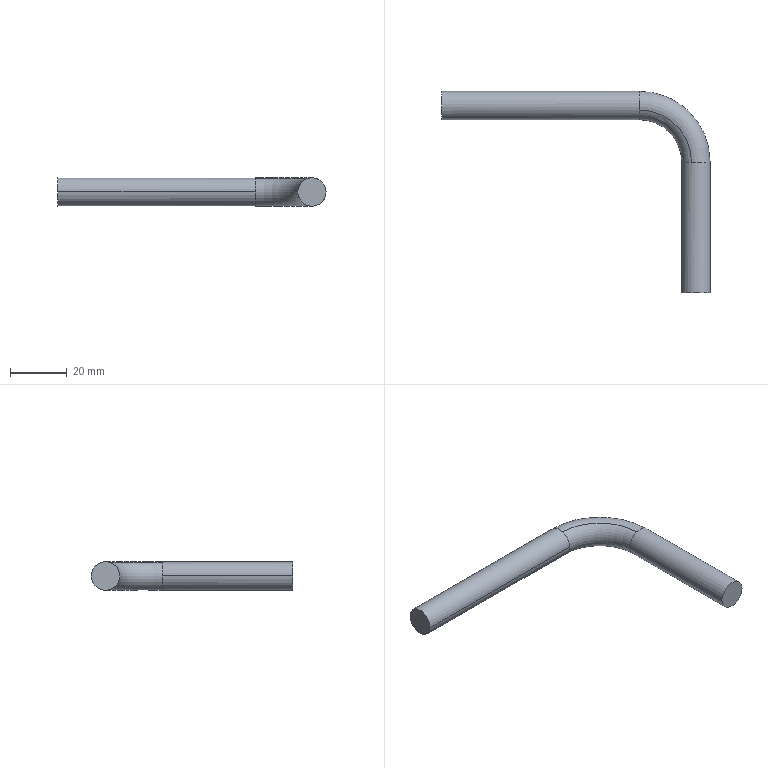Part | 1 solid | 8 faces | box 94.634 x 71 x 10 mm | volume 11549 mm3 | cylinder 4 | plane 2 | torus 2 | commonest cylinder face diameters 10 x4
STEP:
#1=CARTESIAN_POINT('',(0.,0.,0.));
#2=DIRECTION('',(0.,0.,1.));
#3=DIRECTION('',(1.,0.,0.));
#4=AXIS2_PLACEMENT_3D('',#1,#2,#3);
#5=CARTESIAN_POINT('',(-437.297,327.55,-281.55));
#6=VERTEX_POINT('',#5);
#7=CARTESIAN_POINT('',(-437.297,281.55,-281.55));
#8=VERTEX_POINT('',#7);
#9=CARTESIAN_POINT('',(-437.297,327.55,-281.55));
#10=DIRECTION('',(0.,-1.,0.));
#11=VECTOR('',#10,1.);
#12=LINE('',#9,#11);
#13=CARTESIAN_POINT('',(-432.297,327.55,-281.55));
#14=DIRECTION('',(0.,-1.,0.));
#15=DIRECTION('',(0.,0.,1.));
#16=AXIS2_PLACEMENT_3D('',#13,#14,#15);
#17=CYLINDRICAL_SURFACE('',#16,5.);
#18=CARTESIAN_POINT('',(1.571,0.));
#19=DIRECTION('',(0.,1.));
#20=VECTOR('',#19,1.);
#21=LINE('',#18,#20);
#22=(GEOMETRIC_REPRESENTATION_CONTEXT(2)PARAMETRIC_REPRESENTATION_CONTEXT()REPRESENTATION_CONTEXT('',''));
#23=DEFINITIONAL_REPRESENTATION('',(#21),#22);
#24=PCURVE('',#17,#23);
#25=CARTESIAN_POINT('',(-432.297,327.55,-281.55));
#26=DIRECTION('',(0.,-1.,0.));
#27=DIRECTION('',(0.,0.,-1.));
#28=AXIS2_PLACEMENT_3D('',#25,#26,#27);
#29=CYLINDRICAL_SURFACE('',#28,5.);
#30=CARTESIAN_POINT('',(4.712,0.));
#31=DIRECTION('',(0.,1.));
#32=VECTOR('',#31,1.);
#33=LINE('',#30,#32);
#34=(GEOMETRIC_REPRESENTATION_CONTEXT(2)PARAMETRIC_REPRESENTATION_CONTEXT()REPRESENTATION_CONTEXT('',''));
#35=DEFINITIONAL_REPRESENTATION('',(#33),#34);
#36=PCURVE('',#29,#35);
#37=SURFACE_CURVE('',#12,(#24,#36),.PCURVE_S1.);
#38=EDGE_CURVE('',#6,#8,#37,.T.);
#39=ORIENTED_EDGE('',*,*,#38,.F.);
#40=CARTESIAN_POINT('',(-430.751,327.55,-286.305));
#41=VERTEX_POINT('',#40);
#42=CARTESIAN_POINT('',(-432.297,327.55,-281.55));
#43=DIRECTION('',(0.,-1.,0.));
#44=DIRECTION('',(1.,0.,0.));
#45=AXIS2_PLACEMENT_3D('',#42,#43,#44);
#46=CIRCLE('',#45,5.);
#47=CARTESIAN_POINT('',(-1.571,0.));
#48=DIRECTION('',(1.,0.));
#49=VECTOR('',#48,1.);
#50=LINE('',#47,#49);
#51=(GEOMETRIC_REPRESENTATION_CONTEXT(2)PARAMETRIC_REPRESENTATION_CONTEXT()REPRESENTATION_CONTEXT('',''));
#52=DEFINITIONAL_REPRESENTATION('',(#50),#51);
#53=PCURVE('',#17,#52);
#54=CARTESIAN_POINT('',(-452.297,327.55,-281.55));
#55=DIRECTION('',(0.,0.,-1.));
#56=DIRECTION('',(-0.7071,-0.7071,0.));
#57=AXIS2_PLACEMENT_3D('',#54,#55,#56);
#58=TOROIDAL_SURFACE('',#57,20.,5.);
#59=CARTESIAN_POINT('',(3.927,6.283));
#60=DIRECTION('',(0.,-1.));
#61=VECTOR('',#60,1.);
#62=LINE('',#59,#61);
#63=(GEOMETRIC_REPRESENTATION_CONTEXT(2)PARAMETRIC_REPRESENTATION_CONTEXT()REPRESENTATION_CONTEXT('',''));
#64=DEFINITIONAL_REPRESENTATION('',(#62),#63);
#65=PCURVE('',#58,#64);
#66=SURFACE_CURVE('',#46,(#53,#65),.PCURVE_S1.);
#67=EDGE_CURVE('',#6,#41,#66,.T.);
#68=ORIENTED_EDGE('',*,*,#67,.T.);
#69=CARTESIAN_POINT('',(-427.297,327.55,-281.55));
#70=VERTEX_POINT('',#69);
#71=CARTESIAN_POINT('',(-432.297,327.55,-281.55));
#72=DIRECTION('',(0.,-1.,0.));
#73=DIRECTION('',(1.,0.,0.));
#74=AXIS2_PLACEMENT_3D('',#71,#72,#73);
#75=CIRCLE('',#74,5.);
#76=CARTESIAN_POINT('',(-1.571,0.));
#77=DIRECTION('',(1.,0.));
#78=VECTOR('',#77,1.);
#79=LINE('',#76,#78);
#80=(GEOMETRIC_REPRESENTATION_CONTEXT(2)PARAMETRIC_REPRESENTATION_CONTEXT()REPRESENTATION_CONTEXT('',''));
#81=DEFINITIONAL_REPRESENTATION('',(#79),#80);
#82=PCURVE('',#17,#81);
#83=CARTESIAN_POINT('',(-452.297,327.55,-281.55));
#84=DIRECTION('',(0.,0.,-1.));
#85=DIRECTION('',(-0.7071,-0.7071,0.));
#86=AXIS2_PLACEMENT_3D('',#83,#84,#85);
#87=TOROIDAL_SURFACE('',#86,20.,5.);
#88=CARTESIAN_POINT('',(3.927,12.566));
#89=DIRECTION('',(0.,-1.));
#90=VECTOR('',#89,1.);
#91=LINE('',#88,#90);
#92=(GEOMETRIC_REPRESENTATION_CONTEXT(2)PARAMETRIC_REPRESENTATION_CONTEXT()REPRESENTATION_CONTEXT('',''));
#93=DEFINITIONAL_REPRESENTATION('',(#91),#92);
#94=PCURVE('',#87,#93);
#95=SURFACE_CURVE('',#75,(#82,#94),.PCURVE_S1.);
#96=EDGE_CURVE('',#41,#70,#95,.T.);
#97=ORIENTED_EDGE('',*,*,#96,.T.);
#98=CARTESIAN_POINT('',(-427.297,281.55,-281.55));
#99=VERTEX_POINT('',#98);
#100=CARTESIAN_POINT('',(-427.297,327.55,-281.55));
#101=DIRECTION('',(0.,-1.,0.));
#102=VECTOR('',#101,1.);
#103=LINE('',#100,#102);
#104=CARTESIAN_POINT('',(4.712,0.));
#105=DIRECTION('',(0.,1.));
#106=VECTOR('',#105,1.);
#107=LINE('',#104,#106);
#108=(GEOMETRIC_REPRESENTATION_CONTEXT(2)PARAMETRIC_REPRESENTATION_CONTEXT()REPRESENTATION_CONTEXT('',''));
#109=DEFINITIONAL_REPRESENTATION('',(#107),#108);
#110=PCURVE('',#17,#109);
#111=CARTESIAN_POINT('',(1.571,0.));
#112=DIRECTION('',(0.,1.));
#113=VECTOR('',#112,1.);
#114=LINE('',#111,#113);
#115=(GEOMETRIC_REPRESENTATION_CONTEXT(2)PARAMETRIC_REPRESENTATION_CONTEXT()REPRESENTATION_CONTEXT('',''));
#116=DEFINITIONAL_REPRESENTATION('',(#114),#115);
#117=PCURVE('',#29,#116);
#118=SURFACE_CURVE('',#103,(#110,#117),.PCURVE_S1.);
#119=EDGE_CURVE('',#70,#99,#118,.T.);
#120=ORIENTED_EDGE('',*,*,#119,.T.);
#121=CARTESIAN_POINT('',(-432.297,281.55,-281.55));
#122=DIRECTION('',(0.,-1.,0.));
#123=DIRECTION('',(1.,0.,0.));
#124=AXIS2_PLACEMENT_3D('',#121,#122,#123);
#125=CIRCLE('',#124,5.);
#126=CARTESIAN_POINT('',(-1.571,46.));
#127=DIRECTION('',(1.,0.));
#128=VECTOR('',#127,1.);
#129=LINE('',#126,#128);
#130=(GEOMETRIC_REPRESENTATION_CONTEXT(2)PARAMETRIC_REPRESENTATION_CONTEXT()REPRESENTATION_CONTEXT('',''));
#131=DEFINITIONAL_REPRESENTATION('',(#129),#130);
#132=PCURVE('',#17,#131);
#133=CARTESIAN_POINT('',(-432.297,281.55,-281.55));
#134=DIRECTION('',(0.,-1.,0.));
#135=DIRECTION('',(1.,0.,0.));
#136=AXIS2_PLACEMENT_3D('',#133,#134,#135);
#137=PLANE('',#136);
#138=CARTESIAN_POINT('',(0.,0.));
#139=DIRECTION('',(1.,0.));
#140=AXIS2_PLACEMENT_2D('',#138,#139);
#141=CIRCLE('',#140,5.);
#142=(GEOMETRIC_REPRESENTATION_CONTEXT(2)PARAMETRIC_REPRESENTATION_CONTEXT()REPRESENTATION_CONTEXT('',''));
#143=DEFINITIONAL_REPRESENTATION('',(#141),#142);
#144=PCURVE('',#137,#143);
#145=SURFACE_CURVE('',#125,(#132,#144),.PCURVE_S1.);
#146=EDGE_CURVE('',#8,#99,#145,.T.);
#147=ORIENTED_EDGE('',*,*,#146,.F.);
#148=EDGE_LOOP('',(#39,#68,#97,#120,#147));
#149=FACE_BOUND('',#148,.T.);
#150=ADVANCED_FACE('',(#149),#17,.T.);
#151=CARTESIAN_POINT('',(-432.297,281.55,-281.55));
#152=DIRECTION('',(0.,-1.,0.));
#153=DIRECTION('',(1.,0.,0.));
#154=AXIS2_PLACEMENT_3D('',#151,#152,#153);
#155=CIRCLE('',#154,5.);
#156=CARTESIAN_POINT('',(0.,0.));
#157=DIRECTION('',(1.,0.));
#158=AXIS2_PLACEMENT_2D('',#156,#157);
#159=CIRCLE('',#158,5.);
#160=(GEOMETRIC_REPRESENTATION_CONTEXT(2)PARAMETRIC_REPRESENTATION_CONTEXT()REPRESENTATION_CONTEXT('',''));
#161=DEFINITIONAL_REPRESENTATION('',(#159),#160);
#162=PCURVE('',#137,#161);
#163=CARTESIAN_POINT('',(1.571,46.));
#164=DIRECTION('',(1.,0.));
#165=VECTOR('',#164,1.);
#166=LINE('',#163,#165);
#167=(GEOMETRIC_REPRESENTATION_CONTEXT(2)PARAMETRIC_REPRESENTATION_CONTEXT()REPRESENTATION_CONTEXT('',''));
#168=DEFINITIONAL_REPRESENTATION('',(#166),#167);
#169=PCURVE('',#29,#168);
#170=SURFACE_CURVE('',#155,(#162,#169),.PCURVE_S1.);
#171=EDGE_CURVE('',#99,#8,#170,.T.);
#172=ORIENTED_EDGE('',*,*,#171,.T.);
#173=ORIENTED_EDGE('',*,*,#146,.T.);
#174=EDGE_LOOP('',(#172,#173));
#175=FACE_BOUND('',#174,.T.);
#176=ADVANCED_FACE('',(#175),#137,.T.);
#177=CARTESIAN_POINT('',(-452.297,346.005,-276.795));
#178=VERTEX_POINT('',#177);
#179=CARTESIAN_POINT('',(-433.842,327.55,-276.795));
#180=VERTEX_POINT('',#179);
#181=CARTESIAN_POINT('',(-452.297,327.55,-276.795));
#182=DIRECTION('',(0.,0.,-1.));
#183=DIRECTION('',(0.,1.,0.));
#184=AXIS2_PLACEMENT_3D('',#181,#182,#183);
#185=CIRCLE('',#184,18.455);
#186=CARTESIAN_POINT('',(2.356,4.398));
#187=DIRECTION('',(1.,0.));
#188=VECTOR('',#187,1.);
#189=LINE('',#186,#188);
#190=(GEOMETRIC_REPRESENTATION_CONTEXT(2)PARAMETRIC_REPRESENTATION_CONTEXT()REPRESENTATION_CONTEXT('',''));
#191=DEFINITIONAL_REPRESENTATION('',(#189),#190);
#192=PCURVE('',#58,#191);
#193=CARTESIAN_POINT('',(2.356,4.398));
#194=DIRECTION('',(1.,0.));
#195=VECTOR('',#194,1.);
#196=LINE('',#193,#195);
#197=(GEOMETRIC_REPRESENTATION_CONTEXT(2)PARAMETRIC_REPRESENTATION_CONTEXT()REPRESENTATION_CONTEXT('',''));
#198=DEFINITIONAL_REPRESENTATION('',(#196),#197);
#199=PCURVE('',#87,#198);
#200=SURFACE_CURVE('',#185,(#192,#199),.PCURVE_S1.);
#201=EDGE_CURVE('',#178,#180,#200,.T.);
#202=ORIENTED_EDGE('',*,*,#201,.F.);
#203=CARTESIAN_POINT('',(-452.297,342.55,-281.55));
#204=VERTEX_POINT('',#203);
#205=CARTESIAN_POINT('',(-452.297,347.55,-281.55));
#206=DIRECTION('',(1.,0.,0.));
#207=DIRECTION('',(0.,-1.,0.));
#208=AXIS2_PLACEMENT_3D('',#205,#206,#207);
#209=CIRCLE('',#208,5.);
#210=CARTESIAN_POINT('',(2.356,9.425));
#211=DIRECTION('',(0.,-1.));
#212=VECTOR('',#211,1.);
#213=LINE('',#210,#212);
#214=(GEOMETRIC_REPRESENTATION_CONTEXT(2)PARAMETRIC_REPRESENTATION_CONTEXT()REPRESENTATION_CONTEXT('',''));
#215=DEFINITIONAL_REPRESENTATION('',(#213),#214);
#216=PCURVE('',#58,#215);
#217=CARTESIAN_POINT('',(-452.297,347.55,-281.55));
#218=DIRECTION('',(-1.,0.,0.));
#219=DIRECTION('',(0.,0.,-1.));
#220=AXIS2_PLACEMENT_3D('',#217,#218,#219);
#221=CYLINDRICAL_SURFACE('',#220,5.);
#222=CARTESIAN_POINT('',(7.854,0.));
#223=DIRECTION('',(-1.,0.));
#224=VECTOR('',#223,1.);
#225=LINE('',#222,#224);
#226=(GEOMETRIC_REPRESENTATION_CONTEXT(2)PARAMETRIC_REPRESENTATION_CONTEXT()REPRESENTATION_CONTEXT('',''));
#227=DEFINITIONAL_REPRESENTATION('',(#225),#226);
#228=PCURVE('',#221,#227);
#229=SURFACE_CURVE('',#209,(#216,#228),.PCURVE_S1.);
#230=EDGE_CURVE('',#178,#204,#229,.T.);
#231=ORIENTED_EDGE('',*,*,#230,.T.);
#232=CARTESIAN_POINT('',(-452.297,349.095,-286.305));
#233=VERTEX_POINT('',#232);
#234=CARTESIAN_POINT('',(-452.297,347.55,-281.55));
#235=DIRECTION('',(1.,0.,0.));
#236=DIRECTION('',(0.,-1.,0.));
#237=AXIS2_PLACEMENT_3D('',#234,#235,#236);
#238=CIRCLE('',#237,5.);
#239=CARTESIAN_POINT('',(2.356,3.142));
#240=DIRECTION('',(0.,-1.));
#241=VECTOR('',#240,1.);
#242=LINE('',#239,#241);
#243=(GEOMETRIC_REPRESENTATION_CONTEXT(2)PARAMETRIC_REPRESENTATION_CONTEXT()REPRESENTATION_CONTEXT('',''));
#244=DEFINITIONAL_REPRESENTATION('',(#242),#243);
#245=PCURVE('',#58,#244);
#246=CARTESIAN_POINT('',(-452.297,347.55,-281.55));
#247=DIRECTION('',(-1.,0.,0.));
#248=DIRECTION('',(0.,0.,1.));
#249=AXIS2_PLACEMENT_3D('',#246,#247,#248);
#250=CYLINDRICAL_SURFACE('',#249,5.);
#251=CARTESIAN_POINT('',(4.712,0.));
#252=DIRECTION('',(-1.,0.));
#253=VECTOR('',#252,1.);
#254=LINE('',#251,#253);
#255=(GEOMETRIC_REPRESENTATION_CONTEXT(2)PARAMETRIC_REPRESENTATION_CONTEXT()REPRESENTATION_CONTEXT('',''));
#256=DEFINITIONAL_REPRESENTATION('',(#254),#255);
#257=PCURVE('',#250,#256);
#258=SURFACE_CURVE('',#238,(#245,#257),.PCURVE_S1.);
#259=EDGE_CURVE('',#204,#233,#258,.T.);
#260=ORIENTED_EDGE('',*,*,#259,.T.);
#261=CARTESIAN_POINT('',(-452.297,327.55,-286.305));
#262=DIRECTION('',(0.,0.,-1.));
#263=DIRECTION('',(0.,1.,0.));
#264=AXIS2_PLACEMENT_3D('',#261,#262,#263);
#265=CIRCLE('',#264,21.545);
#266=CARTESIAN_POINT('',(2.356,1.257));
#267=DIRECTION('',(1.,0.));
#268=VECTOR('',#267,1.);
#269=LINE('',#266,#268);
#270=(GEOMETRIC_REPRESENTATION_CONTEXT(2)PARAMETRIC_REPRESENTATION_CONTEXT()REPRESENTATION_CONTEXT('',''));
#271=DEFINITIONAL_REPRESENTATION('',(#269),#270);
#272=PCURVE('',#58,#271);
#273=CARTESIAN_POINT('',(2.356,7.54));
#274=DIRECTION('',(1.,0.));
#275=VECTOR('',#274,1.);
#276=LINE('',#273,#275);
#277=(GEOMETRIC_REPRESENTATION_CONTEXT(2)PARAMETRIC_REPRESENTATION_CONTEXT()REPRESENTATION_CONTEXT('',''));
#278=DEFINITIONAL_REPRESENTATION('',(#276),#277);
#279=PCURVE('',#87,#278);
#280=SURFACE_CURVE('',#265,(#272,#279),.PCURVE_S1.);
#281=EDGE_CURVE('',#233,#41,#280,.T.);
#282=ORIENTED_EDGE('',*,*,#281,.T.);
#283=ORIENTED_EDGE('',*,*,#67,.F.);
#284=CARTESIAN_POINT('',(-432.297,327.55,-281.55));
#285=DIRECTION('',(0.,-1.,0.));
#286=DIRECTION('',(1.,0.,0.));
#287=AXIS2_PLACEMENT_3D('',#284,#285,#286);
#288=CIRCLE('',#287,5.);
#289=CARTESIAN_POINT('',(3.927,6.283));
#290=DIRECTION('',(0.,-1.));
#291=VECTOR('',#290,1.);
#292=LINE('',#289,#291);
#293=(GEOMETRIC_REPRESENTATION_CONTEXT(2)PARAMETRIC_REPRESENTATION_CONTEXT()REPRESENTATION_CONTEXT('',''));
#294=DEFINITIONAL_REPRESENTATION('',(#292),#293);
#295=PCURVE('',#58,#294);
#296=CARTESIAN_POINT('',(1.571,0.));
#297=DIRECTION('',(1.,0.));
#298=VECTOR('',#297,1.);
#299=LINE('',#296,#298);
#300=(GEOMETRIC_REPRESENTATION_CONTEXT(2)PARAMETRIC_REPRESENTATION_CONTEXT()REPRESENTATION_CONTEXT('',''));
#301=DEFINITIONAL_REPRESENTATION('',(#299),#300);
#302=PCURVE('',#29,#301);
#303=SURFACE_CURVE('',#288,(#295,#302),.PCURVE_S1.);
#304=EDGE_CURVE('',#180,#6,#303,.T.);
#305=ORIENTED_EDGE('',*,*,#304,.F.);
#306=EDGE_LOOP('',(#202,#231,#260,#282,#283,#305));
#307=FACE_BOUND('',#306,.T.);
#308=ADVANCED_FACE('',(#307),#58,.T.);
#309=CARTESIAN_POINT('',(-452.297,352.55,-281.55));
#310=VERTEX_POINT('',#309);
#311=CARTESIAN_POINT('',(-521.931,352.55,-281.55));
#312=VERTEX_POINT('',#311);
#313=CARTESIAN_POINT('',(-452.297,352.55,-281.55));
#314=DIRECTION('',(-1.,0.,0.));
#315=VECTOR('',#314,1.);
#316=LINE('',#313,#315);
#317=CARTESIAN_POINT('',(1.571,0.));
#318=DIRECTION('',(0.,1.));
#319=VECTOR('',#318,1.);
#320=LINE('',#317,#319);
#321=(GEOMETRIC_REPRESENTATION_CONTEXT(2)PARAMETRIC_REPRESENTATION_CONTEXT()REPRESENTATION_CONTEXT('',''));
#322=DEFINITIONAL_REPRESENTATION('',(#320),#321);
#323=PCURVE('',#250,#322);
#324=CARTESIAN_POINT('',(4.712,0.));
#325=DIRECTION('',(0.,1.));
#326=VECTOR('',#325,1.);
#327=LINE('',#324,#326);
#328=(GEOMETRIC_REPRESENTATION_CONTEXT(2)PARAMETRIC_REPRESENTATION_CONTEXT()REPRESENTATION_CONTEXT('',''));
#329=DEFINITIONAL_REPRESENTATION('',(#327),#328);
#330=PCURVE('',#221,#329);
#331=SURFACE_CURVE('',#316,(#323,#330),.PCURVE_S1.);
#332=EDGE_CURVE('',#310,#312,#331,.T.);
#333=ORIENTED_EDGE('',*,*,#332,.F.);
#334=CARTESIAN_POINT('',(-452.297,347.55,-281.55));
#335=DIRECTION('',(1.,0.,0.));
#336=DIRECTION('',(0.,-1.,0.));
#337=AXIS2_PLACEMENT_3D('',#334,#335,#336);
#338=CIRCLE('',#337,5.);
#339=CARTESIAN_POINT('',(4.712,0.));
#340=DIRECTION('',(-1.,0.));
#341=VECTOR('',#340,1.);
#342=LINE('',#339,#341);
#343=(GEOMETRIC_REPRESENTATION_CONTEXT(2)PARAMETRIC_REPRESENTATION_CONTEXT()REPRESENTATION_CONTEXT('',''));
#344=DEFINITIONAL_REPRESENTATION('',(#342),#343);
#345=PCURVE('',#250,#344);
#346=CARTESIAN_POINT('',(2.356,9.425));
#347=DIRECTION('',(0.,-1.));
#348=VECTOR('',#347,1.);
#349=LINE('',#346,#348);
#350=(GEOMETRIC_REPRESENTATION_CONTEXT(2)PARAMETRIC_REPRESENTATION_CONTEXT()REPRESENTATION_CONTEXT('',''));
#351=DEFINITIONAL_REPRESENTATION('',(#349),#350);
#352=PCURVE('',#87,#351);
#353=SURFACE_CURVE('',#338,(#345,#352),.PCURVE_S1.);
#354=EDGE_CURVE('',#233,#310,#353,.T.);
#355=ORIENTED_EDGE('',*,*,#354,.F.);
#356=ORIENTED_EDGE('',*,*,#259,.F.);
#357=CARTESIAN_POINT('',(-521.931,342.55,-281.55));
#358=VERTEX_POINT('',#357);
#359=CARTESIAN_POINT('',(-452.297,342.55,-281.55));
#360=DIRECTION('',(-1.,0.,0.));
#361=VECTOR('',#360,1.);
#362=LINE('',#359,#361);
#363=CARTESIAN_POINT('',(4.712,0.));
#364=DIRECTION('',(0.,1.));
#365=VECTOR('',#364,1.);
#366=LINE('',#363,#365);
#367=(GEOMETRIC_REPRESENTATION_CONTEXT(2)PARAMETRIC_REPRESENTATION_CONTEXT()REPRESENTATION_CONTEXT('',''));
#368=DEFINITIONAL_REPRESENTATION('',(#366),#367);
#369=PCURVE('',#250,#368);
#370=CARTESIAN_POINT('',(1.571,0.));
#371=DIRECTION('',(0.,1.));
#372=VECTOR('',#371,1.);
#373=LINE('',#370,#372);
#374=(GEOMETRIC_REPRESENTATION_CONTEXT(2)PARAMETRIC_REPRESENTATION_CONTEXT()REPRESENTATION_CONTEXT('',''));
#375=DEFINITIONAL_REPRESENTATION('',(#373),#374);
#376=PCURVE('',#221,#375);
#377=SURFACE_CURVE('',#362,(#369,#376),.PCURVE_S1.);
#378=EDGE_CURVE('',#204,#358,#377,.T.);
#379=ORIENTED_EDGE('',*,*,#378,.T.);
#380=CARTESIAN_POINT('',(-521.931,347.55,-281.55));
#381=DIRECTION('',(1.,0.,0.));
#382=DIRECTION('',(0.,-1.,0.));
#383=AXIS2_PLACEMENT_3D('',#380,#381,#382);
#384=CIRCLE('',#383,5.);
#385=CARTESIAN_POINT('',(4.712,69.634));
#386=DIRECTION('',(-1.,0.));
#387=VECTOR('',#386,1.);
#388=LINE('',#385,#387);
#389=(GEOMETRIC_REPRESENTATION_CONTEXT(2)PARAMETRIC_REPRESENTATION_CONTEXT()REPRESENTATION_CONTEXT('',''));
#390=DEFINITIONAL_REPRESENTATION('',(#388),#389);
#391=PCURVE('',#250,#390);
#392=CARTESIAN_POINT('',(-521.931,347.55,-281.55));
#393=DIRECTION('',(1.,0.,0.));
#394=DIRECTION('',(0.,1.,0.));
#395=AXIS2_PLACEMENT_3D('',#392,#393,#394);
#396=PLANE('',#395);
#397=CARTESIAN_POINT('',(0.,0.));
#398=DIRECTION('',(-1.,0.));
#399=AXIS2_PLACEMENT_2D('',#397,#398);
#400=CIRCLE('',#399,5.);
#401=(GEOMETRIC_REPRESENTATION_CONTEXT(2)PARAMETRIC_REPRESENTATION_CONTEXT()REPRESENTATION_CONTEXT('',''));
#402=DEFINITIONAL_REPRESENTATION('',(#400),#401);
#403=PCURVE('',#396,#402);
#404=SURFACE_CURVE('',#384,(#391,#403),.PCURVE_S1.);
#405=EDGE_CURVE('',#358,#312,#404,.T.);
#406=ORIENTED_EDGE('',*,*,#405,.T.);
#407=EDGE_LOOP('',(#333,#355,#356,#379,#406));
#408=FACE_BOUND('',#407,.T.);
#409=ADVANCED_FACE('',(#408),#250,.T.);
#410=CARTESIAN_POINT('',(-521.931,347.55,-281.55));
#411=DIRECTION('',(1.,0.,0.));
#412=DIRECTION('',(0.,-1.,0.));
#413=AXIS2_PLACEMENT_3D('',#410,#411,#412);
#414=CIRCLE('',#413,5.);
#415=CARTESIAN_POINT('',(0.,0.));
#416=DIRECTION('',(-1.,0.));
#417=AXIS2_PLACEMENT_2D('',#415,#416);
#418=CIRCLE('',#417,5.);
#419=(GEOMETRIC_REPRESENTATION_CONTEXT(2)PARAMETRIC_REPRESENTATION_CONTEXT()REPRESENTATION_CONTEXT('',''));
#420=DEFINITIONAL_REPRESENTATION('',(#418),#419);
#421=PCURVE('',#396,#420);
#422=CARTESIAN_POINT('',(7.854,69.634));
#423=DIRECTION('',(-1.,0.));
#424=VECTOR('',#423,1.);
#425=LINE('',#422,#424);
#426=(GEOMETRIC_REPRESENTATION_CONTEXT(2)PARAMETRIC_REPRESENTATION_CONTEXT()REPRESENTATION_CONTEXT('',''));
#427=DEFINITIONAL_REPRESENTATION('',(#425),#426);
#428=PCURVE('',#221,#427);
#429=SURFACE_CURVE('',#414,(#421,#428),.PCURVE_S1.);
#430=EDGE_CURVE('',#312,#358,#429,.T.);
#431=ORIENTED_EDGE('',*,*,#430,.F.);
#432=ORIENTED_EDGE('',*,*,#405,.F.);
#433=EDGE_LOOP('',(#431,#432));
#434=FACE_BOUND('',#433,.T.);
#435=ADVANCED_FACE('',(#434),#396,.F.);
#436=ORIENTED_EDGE('',*,*,#38,.T.);
#437=ORIENTED_EDGE('',*,*,#171,.F.);
#438=ORIENTED_EDGE('',*,*,#119,.F.);
#439=CARTESIAN_POINT('',(-432.297,327.55,-281.55));
#440=DIRECTION('',(0.,-1.,0.));
#441=DIRECTION('',(1.,0.,0.));
#442=AXIS2_PLACEMENT_3D('',#439,#440,#441);
#443=CIRCLE('',#442,5.);
#444=CARTESIAN_POINT('',(1.571,0.));
#445=DIRECTION('',(1.,0.));
#446=VECTOR('',#445,1.);
#447=LINE('',#444,#446);
#448=(GEOMETRIC_REPRESENTATION_CONTEXT(2)PARAMETRIC_REPRESENTATION_CONTEXT()REPRESENTATION_CONTEXT('',''));
#449=DEFINITIONAL_REPRESENTATION('',(#447),#448);
#450=PCURVE('',#29,#449);
#451=CARTESIAN_POINT('',(3.927,6.283));
#452=DIRECTION('',(0.,-1.));
#453=VECTOR('',#452,1.);
#454=LINE('',#451,#453);
#455=(GEOMETRIC_REPRESENTATION_CONTEXT(2)PARAMETRIC_REPRESENTATION_CONTEXT()REPRESENTATION_CONTEXT('',''));
#456=DEFINITIONAL_REPRESENTATION('',(#454),#455);
#457=PCURVE('',#87,#456);
#458=SURFACE_CURVE('',#443,(#450,#457),.PCURVE_S1.);
#459=EDGE_CURVE('',#70,#180,#458,.T.);
#460=ORIENTED_EDGE('',*,*,#459,.T.);
#461=ORIENTED_EDGE('',*,*,#304,.T.);
#462=EDGE_LOOP('',(#436,#437,#438,#460,#461));
#463=FACE_BOUND('',#462,.T.);
#464=ADVANCED_FACE('',(#463),#29,.T.);
#465=ORIENTED_EDGE('',*,*,#201,.T.);
#466=ORIENTED_EDGE('',*,*,#459,.F.);
#467=ORIENTED_EDGE('',*,*,#96,.F.);
#468=ORIENTED_EDGE('',*,*,#281,.F.);
#469=ORIENTED_EDGE('',*,*,#354,.T.);
#470=CARTESIAN_POINT('',(-452.297,347.55,-281.55));
#471=DIRECTION('',(1.,0.,0.));
#472=DIRECTION('',(0.,-1.,0.));
#473=AXIS2_PLACEMENT_3D('',#470,#471,#472);
#474=CIRCLE('',#473,5.);
#475=CARTESIAN_POINT('',(2.356,9.425));
#476=DIRECTION('',(0.,-1.));
#477=VECTOR('',#476,1.);
#478=LINE('',#475,#477);
#479=(GEOMETRIC_REPRESENTATION_CONTEXT(2)PARAMETRIC_REPRESENTATION_CONTEXT()REPRESENTATION_CONTEXT('',''));
#480=DEFINITIONAL_REPRESENTATION('',(#478),#479);
#481=PCURVE('',#87,#480);
#482=CARTESIAN_POINT('',(7.854,0.));
#483=DIRECTION('',(-1.,0.));
#484=VECTOR('',#483,1.);
#485=LINE('',#482,#484);
#486=(GEOMETRIC_REPRESENTATION_CONTEXT(2)PARAMETRIC_REPRESENTATION_CONTEXT()REPRESENTATION_CONTEXT('',''));
#487=DEFINITIONAL_REPRESENTATION('',(#485),#486);
#488=PCURVE('',#221,#487);
#489=SURFACE_CURVE('',#474,(#481,#488),.PCURVE_S1.);
#490=EDGE_CURVE('',#310,#178,#489,.T.);
#491=ORIENTED_EDGE('',*,*,#490,.T.);
#492=EDGE_LOOP('',(#465,#466,#467,#468,#469,#491));
#493=FACE_BOUND('',#492,.T.);
#494=ADVANCED_FACE('',(#493),#87,.T.);
#495=ORIENTED_EDGE('',*,*,#332,.T.);
#496=ORIENTED_EDGE('',*,*,#430,.T.);
#497=ORIENTED_EDGE('',*,*,#378,.F.);
#498=ORIENTED_EDGE('',*,*,#230,.F.);
#499=ORIENTED_EDGE('',*,*,#490,.F.);
#500=EDGE_LOOP('',(#495,#496,#497,#498,#499));
#501=FACE_BOUND('',#500,.T.);
#502=ADVANCED_FACE('',(#501),#221,.T.);
#503=CLOSED_SHELL('',(#150,#176,#308,#409,#435,#464,#494,#502));
#504=MANIFOLD_SOLID_BREP('',#503);
#505=(LENGTH_UNIT()NAMED_UNIT(*)SI_UNIT(.MILLI.,.METRE.));
#506=UNCERTAINTY_MEASURE_WITH_UNIT(LENGTH_MEASURE(0.0000001),#505,'','');
#507=(NAMED_UNIT(*)PLANE_ANGLE_UNIT()SI_UNIT($,.RADIAN.));
#508=(NAMED_UNIT(*)SI_UNIT($,.STERADIAN.)SOLID_ANGLE_UNIT());
#509=(GEOMETRIC_REPRESENTATION_CONTEXT(3)GLOBAL_UNCERTAINTY_ASSIGNED_CONTEXT((#506))GLOBAL_UNIT_ASSIGNED_CONTEXT((#505,#507,#508))REPRESENTATION_CONTEXT('',''));
#510=ADVANCED_BREP_SHAPE_REPRESENTATION('',(#4,#504),#509);